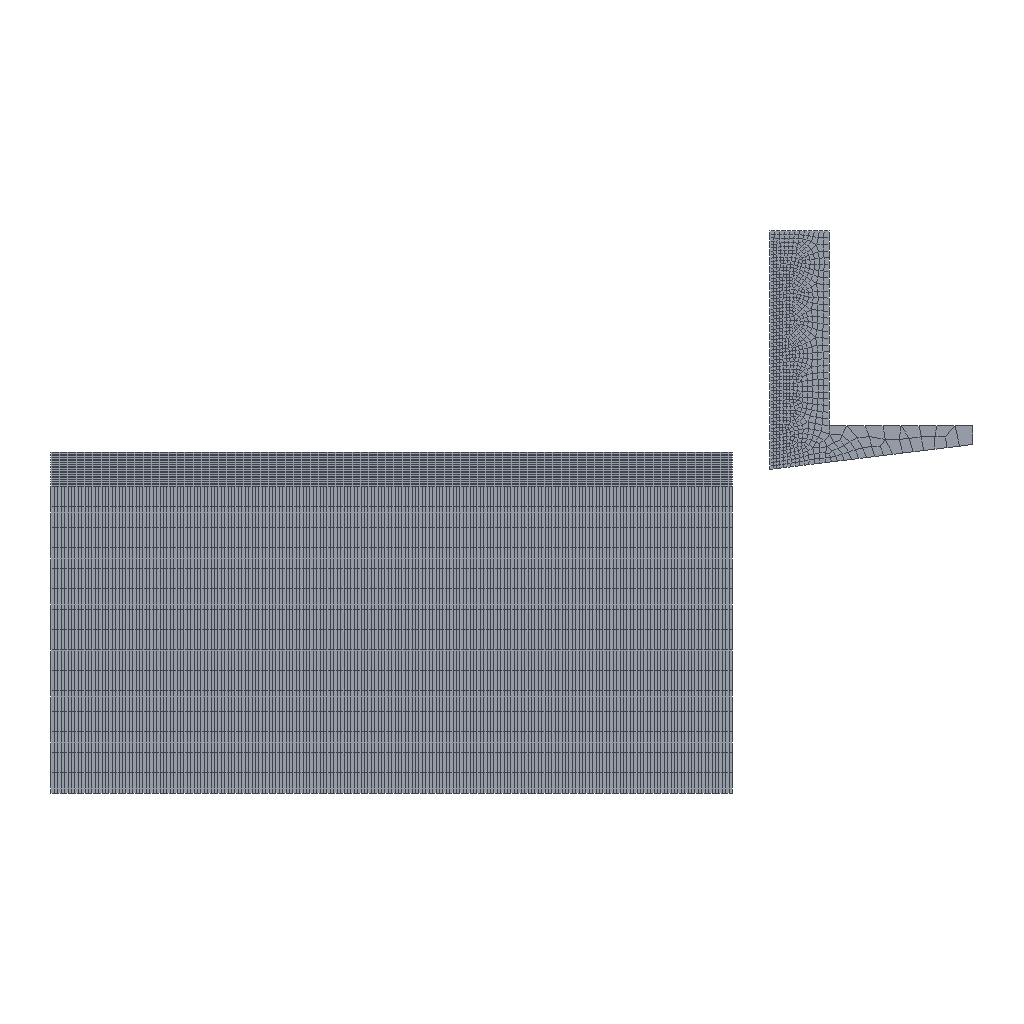Simulation study | abaqus
Set-up summary:
category,name,step,type,value,unit,region
solver,abaqus
solver,version,,,Abaqus/Explicit 2020
units,not stated in the deck,,not stated
analysis,deck,,transient,transient
load_step,Step-1,Step-1,transient
load_step,requested,,,1
mesh,nodes,,,8200
mesh,elements,,,7893
element_type,CPE3T,,plane,11
element_type,CPE4RT,,plane,7882
load,load commands in deck,,count,2
bc,support commands in deck,,count,4
material,TOOL,,in results
material,WORK,,in results
check,setup vs results,,match,"per instance, exact: element labels, types and connectivity; labels of the nodes the elements use; coordinates of those nodes at DOUBLE_PRECISION in 1 of 3 instance(s)"
Abaqus input file, long lists of numbers shortened:
*Heading
** Job name: Job-1 Model name: Model-1
** Generated by: Abaqus/CAE 2020
*Preprint, echo=NO, model=NO, history=NO, contact=NO
**
** PARTS
**
*Part, name=ganggang
*End Part
**
*Part, name=tool
*Node
      1,     0.01734, 0.06212
      2,     0.01734, 0.0562
** (961 more lines like these left out)
*Element, type=CPE3T
 1, 912,  33,  42
 2, 649, 555, 557
** (9 more lines like these left out)
*Element, type=CPE4RT
 12, 272,  58,  57, 271
 13,   1,  56, 256,  53
** (880 more lines like these left out)
*Nset, nset=Set-33, generate
   1,  963,    1
*Elset, elset=Set-33, generate
   1,  893,    1
*Nset, nset=tool-T, generate
   1,  963,    1
*Elset, elset=tool-T, generate
   1,  893,    1
*Elset, elset=_tool-cong_S2, internal
 12, 20, 21, 22, 23, 26, 66, 72, 80, 87, 91, 93
*Elset, elset=_tool-cong_S1, internal
  13,  54,  73,  78,  82,  84,  86,  88, 172, 173
*Elset, elset=_tool-cong_S4, internal
  27,  35,  36,  37,  41,  64,  81,  83,  85,  89,  90,  92, 245, 259, 455
*Surface, type=ELEMENT, name=tool-cong
_tool-cong_S2, S2
_tool-cong_S1, S1
_tool-cong_S4, S4
*Elset, elset=_tool-surf_S1, internal
  17,  30,  32,  33,  44,  47,  49,  56,  57,  63,  68,  70,  76,  94, 103, 104
 109, 110, 111, 114, 115, 116, 120, 121, 122, 126, 127, 128, 131, 132, 133, 137
** (2 more lines like these left out)
*Elset, elset=_tool-surf_S2, internal
  62, 103
*Elset, elset=_tool-surf_S3, internal
  53,  54,  58,  59,  60,  61,  69,  71, 105, 107, 108, 112, 113, 118, 119, 124
 125, 130, 135, 136, 141, 146, 151, 155, 156, 158, 160, 161, 163, 164, 165, 167
** (1 more lines like these left out)
*Elset, elset=_tool-surf_S4, internal
  65,  94, 171, 175, 229
*Surface, type=ELEMENT, name=tool-surf
_tool-surf_S1, S1
_tool-surf_S2, S2
_tool-surf_S4, S4
_tool-surf_S3, S3
** Section: tool
*Solid Section, elset=Set-33, material=tool
,
*End Part
**
*Part, name=work
*Node
      1,           0., -0.01
      2, -0.2, -0.01
** (7234 more lines like these left out)
*Element, type=CPE4RT
   1,    1,    7,  670,  432
   2,    7,    8,  671,  670
** (6998 more lines like these left out)
*Nset, nset=Set-1, generate
    1,  7236,     1
*Elset, elset=Set-1, generate
    1,  7000,     1
*Nset, nset=chipaa
    5,    6,  435,  436,  437,  438,  439,  440,  441,  442,  443,  444,  445,  446,  447,  448
  449,  450,  451,  452,  453,  454,  455,  456,  457,  458,  459,  460,  461,  462,  463,  464
** (225 more lines like these left out)
** Section: work
*Solid Section, elset=Set-1, material=work
,
*End Part
**
**
** ASSEMBLY
**
*Assembly, name=Assembly
**
*Instance, name=tool-1, part=tool
       0.011,       -0.005,           0.
*End Instance
**
*Instance, name=work-1, part=work
*End Instance
**
*Instance, name=ganggang-1, part=ganggang
    0.000337,     0.4978,           0.
*Node
      1,  0.428,  0.11,           0.
*Nset, nset=ganggang-1-RefPt_, internal
1,
*Surface, type=SEGMENTS, name=gang-zhu
START,        0.028,        -0.49
 LINE,        0.028,         0.11
 LINE,        0.428,         0.11
 LINE,        0.428,        -0.49
 LINE,        0.028,        -0.49
*Rigid Body, ref node=ganggang-1-RefPt_, analytical surface=gang-zhu
*End Instance
**
*Nset, nset=Set-2, instance=work-1
   1,   2,   3,   4, 206, 207, 208, 209, 210, 211, 212, 213, 214, 215, 216, 217
 218, 219, 220, 221, 222, 223, 224, 225, 226, 227, 228, 229, 230, 231, 232, 233
** (13 more lines like these left out)
*Elset, elset=Set-2, instance=work-1
    1,  200,  201,  400,  401,  600,  601,  800,  801, 1000, 1001, 1200, 1201, 1400, 1401, 1600
 1601, 1800, 1801, 2000, 2001, 2200, 2201, 2400, 2401, 2600, 2601, 2800, 2801, 2802, 2803, 2804
** (13 more lines like these left out)
*Nset, nset=Set-5, instance=work-1, generate
    1,  7236,     1
*Elset, elset=Set-5, instance=work-1, generate
    1,  7000,     1
*Nset, nset=Set-9, instance=ganggang-1
 1,
*Nset, nset=Set-10, instance=ganggang-1
 1,
*Nset, nset=Set-11, instance=tool-1, generate
   1,  963,    1
*Elset, elset=Set-11, instance=tool-1, generate
   1,  893,    1
*Nset, nset=Set-12, instance=tool-1, generate
   1,  963,    1
*Elset, elset=Set-12, instance=tool-1, generate
   1,  893,    1
*Nset, nset=Set-13, instance=work-1
   3,   4, 220, 221, 222, 223, 224, 225, 226, 227, 228, 229, 230, 231, 232, 233
 234, 235, 236, 237, 238, 239, 240, 241, 242, 243, 244, 245, 246, 247, 248, 249
** (11 more lines like these left out)
*Elset, elset=Set-13, instance=work-1, generate
 2801,  3000,     1
*Nset, nset=Set-14, instance=work-1
   1,   2,   3,   4, 206, 207, 208, 209, 210, 211, 212, 213, 214, 215, 216, 217
 218, 219, 220, 221, 222, 223, 224, 225, 226, 227, 228, 229, 230, 231, 232, 233
** (13 more lines like these left out)
*Elset, elset=Set-14, instance=work-1
    1,  200,  201,  400,  401,  600,  601,  800,  801, 1000, 1001, 1200, 1201, 1400, 1401, 1600
 1601, 1800, 1801, 2000, 2001, 2200, 2201, 2400, 2401, 2600, 2601, 2800, 2801, 2802, 2803, 2804
** (13 more lines like these left out)
*Nset, nset=Set-18, instance=work-1
   1,   2,   3,   4, 206, 207, 208, 209, 210, 211, 212, 213, 214, 215, 216, 217
 218, 219, 220, 221, 222, 223, 224, 225, 226, 227, 228, 229, 230, 231, 232, 233
** (13 more lines like these left out)
*Elset, elset=Set-18, instance=work-1
    1,  200,  201,  400,  401,  600,  601,  800,  801, 1000, 1001, 1200, 1201, 1400, 1401, 1600
 1601, 1800, 1801, 2000, 2001, 2200, 2201, 2400, 2401, 2600, 2601, 2800, 2801, 2802, 2803, 2804
** (13 more lines like these left out)
*Nset, nset=Set-20, instance=tool-1
   1,   2,   3,   4,   5,   6,   7,   8,   9,  29,  30,  31,  32,  33,  34,  35
  54,  55,  56,  57,  58,  59,  60,  61,  62,  63,  64,  65,  66,  67,  68,  69
** (1 more lines like these left out)
*Elset, elset=Set-20, instance=tool-1
  12,  13,  20,  21,  22,  23,  26,  27,  35,  36,  37,  41,  54,  64,  66,  72
  73,  78,  80,  81,  82,  83,  84,  85,  86,  87,  88,  89,  90,  91,  92,  93
** (1 more lines like these left out)
*Nset, nset=Set-21, instance=tool-1
   1,   2,   3,   4,   5,   6,   7,   8,   9,  29,  30,  31,  32,  33,  34,  35
  54,  55,  56,  57,  58,  59,  60,  61,  62,  63,  64,  65,  66,  67,  68,  69
** (1 more lines like these left out)
*Elset, elset=Set-21, instance=tool-1
  12,  13,  20,  21,  22,  23,  26,  27,  35,  36,  37,  41,  54,  64,  66,  72
  73,  78,  80,  81,  82,  83,  84,  85,  86,  87,  88,  89,  90,  91,  92,  93
** (1 more lines like these left out)
*Nset, nset=Set-22, instance=ganggang-1
 1,
*Nset, nset=Set-23, instance=ganggang-1
 1,
*Nset, nset=_PickedSet23, internal, instance=work-1
    1,    2,    5,    6,    7,    8,    9,   10,   11,   12,   13,   14,   15,   16,   17,   18
   19,   20,   21,   22,   23,   24,   25,   26,   27,   28,   29,   30,   31,   32,   33,   34
** (262 more lines like these left out)
*Elset, elset=_PickedSet23, internal, instance=work-1, generate
 3001,  7000,     1
*Elset, elset=_s_Surf-1_S2, internal, instance=tool-1
  62,  78, 100, 103, 238, 239
*Elset, elset=_s_Surf-1_S4, internal, instance=tool-1
  54,  65,  94,  98,  99, 102, 171, 175, 228, 229, 244
*Elset, elset=_s_Surf-1_S3, internal, instance=tool-1
  53,  54,  58,  59,  60,  61,  69,  71, 101, 160, 161, 163, 164, 165, 167, 169
*Elset, elset=_s_Surf-1_S1, internal, instance=tool-1
  57,  63,  76, 104, 170, 174, 234, 271, 884
*Surface, type=ELEMENT, name=s_Surf-1
_s_Surf-1_S2, S2
_s_Surf-1_S4, S4
_s_Surf-1_S3, S3
_s_Surf-1_S1, S1
*Elset, elset=_s_Surf-2_S2, internal, instance=tool-1
 12, 20, 21, 22, 23, 26, 66, 72, 80, 87, 91, 93
*Elset, elset=_s_Surf-2_S1, internal, instance=tool-1
  13,  54,  73,  78,  82,  84,  86,  88, 172, 173
*Elset, elset=_s_Surf-2_S4, internal, instance=tool-1
  27,  35,  36,  37,  41,  64,  81,  83,  85,  89,  90,  92, 245, 259, 455
*Surface, type=ELEMENT, name=s_Surf-2
_s_Surf-2_S2, S2
_s_Surf-2_S1, S1
_s_Surf-2_S4, S4
*Elset, elset=_s_Surf-4_S2, internal, instance=tool-1
  12,  20,  21,  22,  23,  26,  66,  72,  78,  80,  87,  91,  93, 100, 238, 239
*Elset, elset=_s_Surf-4_S1, internal, instance=tool-1
  13,  54,  73,  78,  82,  84,  86,  88, 172, 173
*Elset, elset=_s_Surf-4_S4, internal, instance=tool-1
  27,  35,  36,  37,  41,  54,  64,  81,  83,  85,  89,  90,  92,  94,  98,  99
 102, 228, 229, 244, 245, 259, 455
*Elset, elset=_s_Surf-4_S3, internal, instance=tool-1
 101,
*Surface, type=ELEMENT, name=s_Surf-4
_s_Surf-4_S2, S2
_s_Surf-4_S1, S1
_s_Surf-4_S4, S4
_s_Surf-4_S3, S3
*Surface, type=NODE, name=work-1_chipaa_CNS_, internal
work-1.chipaa, 1.
** Constraint: Constraint-1
*Tie, name=Constraint-1, adjust=yes, type=SURFACE TO SURFACE
tool-1.tool-cong, ganggang-1.gang-zhu
*End Assembly
*Amplitude, name=Amp-1, definition=PERIODIC
1,         213520.,              0.,              0.
         427.04,              0.
*Amplitude, name=Amp-2
             0.,              0.,           0.003,             0.1,           0.005,             0.4,           0.007,             0.7
           0.01,              1.
**
** MATERIALS
**
*Material, name=tool
*Conductivity
2000.,
*Density
 3.51e-09,
*Elastic
 1e+06, 0.2
*Specific Heat
 5.079e+08,
*Material, name=work
*Conductivity
173.,
*Damage Initiation, criterion=JOHNSON COOK
0.,  0.33,  -1.5, 0.042,    0., 3397.,   20.,    1.
*Damage Evolution, type=DISPLACEMENT
 0.001,
*Density
 1.76e-08,
*Elastic
314000., 0.28
*Inelastic Heat Fraction
         0.9,
*Plastic, hardening=JOHNSON COOK
 1505.8, 176.5,  0.12,    1., 3397.,   20.
*Rate Dependent, type=JOHNSON COOK
 0.016,1.
*Specific Heat
 3.84e+08,
**
** INTERACTION PROPERTIES
**
*Surface Interaction, name=IntProp-1
*Friction
 0.3,
*Surface Behavior, pressure-overclosure=HARD
**
** PREDEFINED FIELDS
**
** Name: Predefined Field-1   Type: Temperature
*Initial Conditions, type=TEMPERATURE
Set-5, 20.
** Name: Predefined Field-2   Type: Temperature
*Initial Conditions, type=TEMPERATURE
tool-1.tool-T, 20.
** ----------------------------------------------------------------
**
** STEP: Step-1
**
*Step, name=Step-1, nlgeom=YES
*Dynamic, Explicit
, 0.012
*Bulk Viscosity
0.06, 1.2
** Mass Scaling: Semi-Automatic
**               Whole Model
*Fixed Mass Scaling, dt=1e-08, type=below min
**
** BOUNDARY CONDITIONS
**
** Name: BC-1 Type: 对称/反对称/完全固定
*Boundary
Set-18, ENCASTRE
** Name: BC-2 Type: 速度/角速度
*Boundary, amplitude=Amp-2, type=VELOCITY
Set-22, 1, 1, -16.67
Set-22, 6, 6
** Name: BC-3 Type: 速度/角速度
*Boundary, amplitude=Amp-1, type=VELOCITY
Set-23, 2, 2, 1.
*Adaptive Mesh Controls, name=Ada-1
1., 0., 0.
**
** INTERACTIONS
**
** Interaction: Int-1
*Contact Pair, interaction=IntProp-1, mechanical constraint=KINEMATIC, cpset=Int-1
tool-1.tool-surf, work-1_chipaa_CNS_
**
** OUTPUT REQUESTS
**
*Restart, write, number interval=1, time marks=NO
**
** FIELD OUTPUT: F-Output-1
**
*Output, field
*Node Output
A, RF, U, V
*Element Output, directions=YES
E, EVF, LE, MISES, PE, PEEQ, PEEQVAVG, PEVAVG, S, STATUS, SVAVG, TEMP
*Contact Output
CSTRESS,
**
** HISTORY OUTPUT: H-Output-1
**
*Output, history, variable=PRESELECT
*End Step
Results summary:
result,step,Step-1,completed,increments=2105071 time=0.012/0.012
result,analysis,,,transient
result,last_loadstep,,,1
result,primary field,,,U
result,reaction total,,FX,1.489,model units
result,reaction total,,FY,25.003,model units
result,reaction total,,FZ,0.0,model units